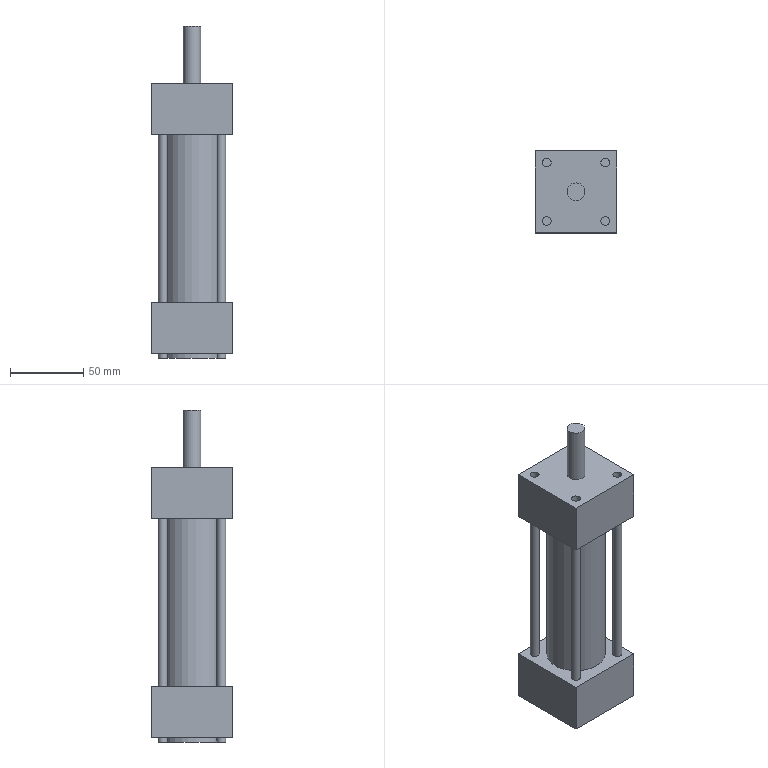Part | NX | features MAIN_BODY 2 | 1 solid | 37 faces | box 56 x 56 x 227 mm | volume 382506 mm3 | plane 22 | cylinder 15 | commonest cylinder face diameters 6.2 x8 6 x4 40 x2 12 x1
STEP:
#1=CARTESIAN_POINT('',(652.5,-160.,-165.));
#2=VERTEX_POINT('',#1);
#3=CARTESIAN_POINT('',(652.5,-140.,-165.));
#4=DIRECTION('',(0.,0.,1.));
#5=DIRECTION('',(0.,-1.,0.));
#6=AXIS2_PLACEMENT_3D('',#3,#4,#5);
#7=CIRCLE('',#6,20.);
#8=EDGE_CURVE('',#2,#2,#7,.T.);
#9=ORIENTED_EDGE('',*,*,#8,.F.);
#10=EDGE_LOOP('',(#9));
#11=FACE_BOUND('',#10,.T.);
#12=CARTESIAN_POINT('',(652.5,-160.,-280.));
#13=VERTEX_POINT('',#12);
#14=CARTESIAN_POINT('',(652.5,-140.,-280.));
#15=DIRECTION('',(0.,0.,1.));
#16=DIRECTION('',(0.,-1.,0.));
#17=AXIS2_PLACEMENT_3D('',#14,#15,#16);
#18=CIRCLE('',#17,20.);
#19=EDGE_CURVE('',#13,#13,#18,.F.);
#20=ORIENTED_EDGE('',*,*,#19,.F.);
#21=EDGE_LOOP('',(#20));
#22=FACE_BOUND('',#21,.T.);
#23=CARTESIAN_POINT('',(652.5,-140.,-315.));
#24=DIRECTION('',(0.,0.,1.));
#25=DIRECTION('',(0.,1.,0.));
#26=AXIS2_PLACEMENT_3D('',#23,#24,#25);
#27=CYLINDRICAL_SURFACE('',#26,20.);
#28=ADVANCED_FACE('',(#11,#22),#27,.T.);
#29=CARTESIAN_POINT('',(632.5,-163.,-130.));
#30=VERTEX_POINT('',#29);
#31=CARTESIAN_POINT('',(632.5,-160.,-130.));
#32=DIRECTION('',(0.,0.,-1.));
#33=DIRECTION('',(0.,-1.,0.));
#34=AXIS2_PLACEMENT_3D('',#31,#32,#33);
#35=CIRCLE('',#34,3.);
#36=EDGE_CURVE('',#30,#30,#35,.T.);
#37=ORIENTED_EDGE('',*,*,#36,.T.);
#38=EDGE_LOOP('',(#37));
#39=FACE_BOUND('',#38,.T.);
#40=CARTESIAN_POINT('',(632.5,-117.,-130.));
#41=VERTEX_POINT('',#40);
#42=CARTESIAN_POINT('',(632.5,-120.,-130.));
#43=DIRECTION('',(0.,0.,1.));
#44=DIRECTION('',(0.,1.,0.));
#45=AXIS2_PLACEMENT_3D('',#42,#43,#44);
#46=CIRCLE('',#45,3.);
#47=EDGE_CURVE('',#41,#41,#46,.T.);
#48=ORIENTED_EDGE('',*,*,#47,.F.);
#49=EDGE_LOOP('',(#48));
#50=FACE_BOUND('',#49,.T.);
#51=CARTESIAN_POINT('',(680.5,-112.,-130.));
#52=VERTEX_POINT('',#51);
#53=CARTESIAN_POINT('',(624.5,-112.,-130.));
#54=VERTEX_POINT('',#53);
#55=CARTESIAN_POINT('',(680.5,-112.,-130.));
#56=DIRECTION('',(-1.,0.,0.));
#57=VECTOR('',#56,1000.);
#58=LINE('',#55,#57);
#59=EDGE_CURVE('',#52,#54,#58,.T.);
#60=ORIENTED_EDGE('',*,*,#59,.T.);
#61=CARTESIAN_POINT('',(624.5,-168.,-130.));
#62=VERTEX_POINT('',#61);
#63=CARTESIAN_POINT('',(624.5,-112.,-130.));
#64=DIRECTION('',(0.,-1.,0.));
#65=VECTOR('',#64,1000.);
#66=LINE('',#63,#65);
#67=EDGE_CURVE('',#54,#62,#66,.T.);
#68=ORIENTED_EDGE('',*,*,#67,.T.);
#69=CARTESIAN_POINT('',(680.5,-168.,-130.));
#70=VERTEX_POINT('',#69);
#71=CARTESIAN_POINT('',(624.5,-168.,-130.));
#72=DIRECTION('',(1.,0.,0.));
#73=VECTOR('',#72,1000.);
#74=LINE('',#71,#73);
#75=EDGE_CURVE('',#62,#70,#74,.T.);
#76=ORIENTED_EDGE('',*,*,#75,.T.);
#77=CARTESIAN_POINT('',(680.5,-168.,-130.));
#78=DIRECTION('',(0.,1.,0.));
#79=VECTOR('',#78,1000.);
#80=LINE('',#77,#79);
#81=EDGE_CURVE('',#70,#52,#80,.T.);
#82=ORIENTED_EDGE('',*,*,#81,.T.);
#83=EDGE_LOOP('',(#60,#68,#76,#82));
#84=FACE_BOUND('',#83,.T.);
#85=CARTESIAN_POINT('',(672.5,-163.,-130.));
#86=VERTEX_POINT('',#85);
#87=CARTESIAN_POINT('',(672.5,-160.,-130.));
#88=DIRECTION('',(0.,0.,1.));
#89=DIRECTION('',(0.,-1.,0.));
#90=AXIS2_PLACEMENT_3D('',#87,#88,#89);
#91=CIRCLE('',#90,3.);
#92=EDGE_CURVE('',#86,#86,#91,.T.);
#93=ORIENTED_EDGE('',*,*,#92,.F.);
#94=EDGE_LOOP('',(#93));
#95=FACE_BOUND('',#94,.T.);
#96=CARTESIAN_POINT('',(672.5,-117.,-130.));
#97=VERTEX_POINT('',#96);
#98=CARTESIAN_POINT('',(672.5,-120.,-130.));
#99=DIRECTION('',(0.,0.,-1.));
#100=DIRECTION('',(0.,1.,0.));
#101=AXIS2_PLACEMENT_3D('',#98,#99,#100);
#102=CIRCLE('',#101,3.);
#103=EDGE_CURVE('',#97,#97,#102,.T.);
#104=ORIENTED_EDGE('',*,*,#103,.T.);
#105=EDGE_LOOP('',(#104));
#106=FACE_BOUND('',#105,.T.);
#107=CARTESIAN_POINT('',(652.5,-146.,-130.));
#108=VERTEX_POINT('',#107);
#109=CARTESIAN_POINT('',(652.5,-140.,-130.));
#110=DIRECTION('',(0.,0.,1.));
#111=DIRECTION('',(0.,-1.,0.));
#112=AXIS2_PLACEMENT_3D('',#109,#110,#111);
#113=CIRCLE('',#112,6.);
#114=EDGE_CURVE('',#108,#108,#113,.F.);
#115=ORIENTED_EDGE('',*,*,#114,.T.);
#116=EDGE_LOOP('',(#115));
#117=FACE_BOUND('',#116,.T.);
#118=CARTESIAN_POINT('',(624.5,-112.,-130.));
#119=DIRECTION('',(0.,0.,-1.));
#120=DIRECTION('',(0.,-1.,0.));
#121=AXIS2_PLACEMENT_3D('',#118,#119,#120);
#122=PLANE('',#121);
#123=ADVANCED_FACE('',(#39,#50,#84,#95,#106,#117),#122,.F.);
#124=ORIENTED_EDGE('',*,*,#59,.F.);
#125=CARTESIAN_POINT('',(680.5,-112.,-165.));
#126=VERTEX_POINT('',#125);
#127=CARTESIAN_POINT('',(680.5,-112.,-165.));
#128=DIRECTION('',(0.,0.,1.));
#129=VECTOR('',#128,1000.);
#130=LINE('',#127,#129);
#131=EDGE_CURVE('',#126,#52,#130,.T.);
#132=ORIENTED_EDGE('',*,*,#131,.F.);
#133=CARTESIAN_POINT('',(624.5,-112.,-165.));
#134=VERTEX_POINT('',#133);
#135=CARTESIAN_POINT('',(680.5,-112.,-165.));
#136=DIRECTION('',(-1.,0.,0.));
#137=VECTOR('',#136,1000.);
#138=LINE('',#135,#137);
#139=EDGE_CURVE('',#126,#134,#138,.T.);
#140=ORIENTED_EDGE('',*,*,#139,.T.);
#141=CARTESIAN_POINT('',(624.5,-112.,-165.));
#142=DIRECTION('',(0.,0.,1.));
#143=VECTOR('',#142,1000.);
#144=LINE('',#141,#143);
#145=EDGE_CURVE('',#134,#54,#144,.T.);
#146=ORIENTED_EDGE('',*,*,#145,.T.);
#147=EDGE_LOOP('',(#124,#132,#140,#146));
#148=FACE_BOUND('',#147,.T.);
#149=CARTESIAN_POINT('',(680.5,-112.,-165.));
#150=DIRECTION('',(0.,-1.,0.));
#151=DIRECTION('',(-1.,0.,0.));
#152=AXIS2_PLACEMENT_3D('',#149,#150,#151);
#153=PLANE('',#152);
#154=ADVANCED_FACE('',(#148),#153,.F.);
#155=ORIENTED_EDGE('',*,*,#67,.F.);
#156=ORIENTED_EDGE('',*,*,#145,.F.);
#157=CARTESIAN_POINT('',(624.5,-168.,-165.));
#158=VERTEX_POINT('',#157);
#159=CARTESIAN_POINT('',(624.5,-112.,-165.));
#160=DIRECTION('',(0.,-1.,0.));
#161=VECTOR('',#160,1000.);
#162=LINE('',#159,#161);
#163=EDGE_CURVE('',#134,#158,#162,.T.);
#164=ORIENTED_EDGE('',*,*,#163,.T.);
#165=CARTESIAN_POINT('',(624.5,-168.,-165.));
#166=DIRECTION('',(0.,0.,1.));
#167=VECTOR('',#166,1000.);
#168=LINE('',#165,#167);
#169=EDGE_CURVE('',#158,#62,#168,.T.);
#170=ORIENTED_EDGE('',*,*,#169,.T.);
#171=EDGE_LOOP('',(#155,#156,#164,#170));
#172=FACE_BOUND('',#171,.T.);
#173=CARTESIAN_POINT('',(624.5,-112.,-165.));
#174=DIRECTION('',(1.,0.,0.));
#175=DIRECTION('',(0.,0.,1.));
#176=AXIS2_PLACEMENT_3D('',#173,#174,#175);
#177=PLANE('',#176);
#178=ADVANCED_FACE('',(#172),#177,.F.);
#179=ORIENTED_EDGE('',*,*,#75,.F.);
#180=ORIENTED_EDGE('',*,*,#169,.F.);
#181=CARTESIAN_POINT('',(680.5,-168.,-165.));
#182=VERTEX_POINT('',#181);
#183=CARTESIAN_POINT('',(624.5,-168.,-165.));
#184=DIRECTION('',(1.,0.,0.));
#185=VECTOR('',#184,1000.);
#186=LINE('',#183,#185);
#187=EDGE_CURVE('',#158,#182,#186,.T.);
#188=ORIENTED_EDGE('',*,*,#187,.T.);
#189=CARTESIAN_POINT('',(680.5,-168.,-165.));
#190=DIRECTION('',(0.,0.,1.));
#191=VECTOR('',#190,1000.);
#192=LINE('',#189,#191);
#193=EDGE_CURVE('',#182,#70,#192,.T.);
#194=ORIENTED_EDGE('',*,*,#193,.T.);
#195=EDGE_LOOP('',(#179,#180,#188,#194));
#196=FACE_BOUND('',#195,.T.);
#197=CARTESIAN_POINT('',(624.5,-168.,-165.));
#198=DIRECTION('',(0.,1.,0.));
#199=DIRECTION('',(0.,0.,-1.));
#200=AXIS2_PLACEMENT_3D('',#197,#198,#199);
#201=PLANE('',#200);
#202=ADVANCED_FACE('',(#196),#201,.F.);
#203=CARTESIAN_POINT('',(632.5,-123.,-165.));
#204=VERTEX_POINT('',#203);
#205=CARTESIAN_POINT('',(632.5,-120.,-165.));
#206=DIRECTION('',(0.,0.,1.));
#207=DIRECTION('',(0.,-1.,0.));
#208=AXIS2_PLACEMENT_3D('',#205,#206,#207);
#209=CIRCLE('',#208,3.);
#210=EDGE_CURVE('',#204,#204,#209,.T.);
#211=ORIENTED_EDGE('',*,*,#210,.F.);
#212=EDGE_LOOP('',(#211));
#213=FACE_BOUND('',#212,.T.);
#214=ORIENTED_EDGE('',*,*,#47,.T.);
#215=EDGE_LOOP('',(#214));
#216=FACE_BOUND('',#215,.T.);
#217=CARTESIAN_POINT('',(632.5,-120.,-165.));
#218=DIRECTION('',(0.,0.,1.));
#219=DIRECTION('',(0.,1.,0.));
#220=AXIS2_PLACEMENT_3D('',#217,#218,#219);
#221=CYLINDRICAL_SURFACE('',#220,3.);
#222=ADVANCED_FACE('',(#213,#216),#221,.F.);
#223=ORIENTED_EDGE('',*,*,#81,.F.);
#224=ORIENTED_EDGE('',*,*,#193,.F.);
#225=CARTESIAN_POINT('',(680.5,-168.,-165.));
#226=DIRECTION('',(0.,1.,0.));
#227=VECTOR('',#226,1000.);
#228=LINE('',#225,#227);
#229=EDGE_CURVE('',#182,#126,#228,.T.);
#230=ORIENTED_EDGE('',*,*,#229,.T.);
#231=ORIENTED_EDGE('',*,*,#131,.T.);
#232=EDGE_LOOP('',(#223,#224,#230,#231));
#233=FACE_BOUND('',#232,.T.);
#234=CARTESIAN_POINT('',(680.5,-168.,-165.));
#235=DIRECTION('',(-1.,0.,0.));
#236=DIRECTION('',(0.,0.,-1.));
#237=AXIS2_PLACEMENT_3D('',#234,#235,#236);
#238=PLANE('',#237);
#239=ADVANCED_FACE('',(#233),#238,.F.);
#240=CARTESIAN_POINT('',(672.5,-163.,-165.));
#241=VERTEX_POINT('',#240);
#242=CARTESIAN_POINT('',(672.5,-160.,-165.));
#243=DIRECTION('',(0.,0.,1.));
#244=DIRECTION('',(0.,-1.,0.));
#245=AXIS2_PLACEMENT_3D('',#242,#243,#244);
#246=CIRCLE('',#245,3.);
#247=EDGE_CURVE('',#241,#241,#246,.T.);
#248=ORIENTED_EDGE('',*,*,#247,.F.);
#249=EDGE_LOOP('',(#248));
#250=FACE_BOUND('',#249,.T.);
#251=ORIENTED_EDGE('',*,*,#92,.T.);
#252=EDGE_LOOP('',(#251));
#253=FACE_BOUND('',#252,.T.);
#254=CARTESIAN_POINT('',(672.5,-160.,-165.));
#255=DIRECTION('',(0.,0.,1.));
#256=DIRECTION('',(0.,1.,0.));
#257=AXIS2_PLACEMENT_3D('',#254,#255,#256);
#258=CYLINDRICAL_SURFACE('',#257,3.);
#259=ADVANCED_FACE('',(#250,#253),#258,.F.);
#260=CARTESIAN_POINT('',(672.5,-117.,-165.));
#261=VERTEX_POINT('',#260);
#262=CARTESIAN_POINT('',(672.5,-120.,-165.));
#263=DIRECTION('',(0.,0.,-1.));
#264=DIRECTION('',(0.,1.,0.));
#265=AXIS2_PLACEMENT_3D('',#262,#263,#264);
#266=CIRCLE('',#265,3.);
#267=EDGE_CURVE('',#261,#261,#266,.T.);
#268=ORIENTED_EDGE('',*,*,#267,.T.);
#269=EDGE_LOOP('',(#268));
#270=FACE_BOUND('',#269,.T.);
#271=ORIENTED_EDGE('',*,*,#103,.F.);
#272=EDGE_LOOP('',(#271));
#273=FACE_BOUND('',#272,.T.);
#274=CARTESIAN_POINT('',(672.5,-120.,-165.));
#275=DIRECTION('',(0.,0.,1.));
#276=DIRECTION('',(0.,1.,0.));
#277=AXIS2_PLACEMENT_3D('',#274,#275,#276);
#278=CYLINDRICAL_SURFACE('',#277,3.);
#279=ADVANCED_FACE('',(#270,#273),#278,.F.);
#280=CARTESIAN_POINT('',(632.5,-163.,-165.));
#281=VERTEX_POINT('',#280);
#282=CARTESIAN_POINT('',(632.5,-160.,-165.));
#283=DIRECTION('',(0.,0.,-1.));
#284=DIRECTION('',(0.,-1.,0.));
#285=AXIS2_PLACEMENT_3D('',#282,#283,#284);
#286=CIRCLE('',#285,3.);
#287=EDGE_CURVE('',#281,#281,#286,.T.);
#288=ORIENTED_EDGE('',*,*,#287,.T.);
#289=EDGE_LOOP('',(#288));
#290=FACE_BOUND('',#289,.T.);
#291=ORIENTED_EDGE('',*,*,#36,.F.);
#292=EDGE_LOOP('',(#291));
#293=FACE_BOUND('',#292,.T.);
#294=CARTESIAN_POINT('',(632.5,-160.,-165.));
#295=DIRECTION('',(0.,0.,1.));
#296=DIRECTION('',(0.,1.,0.));
#297=AXIS2_PLACEMENT_3D('',#294,#295,#296);
#298=CYLINDRICAL_SURFACE('',#297,3.);
#299=ADVANCED_FACE('',(#290,#293),#298,.F.);
#300=CARTESIAN_POINT('',(632.5,-123.1,-165.));
#301=VERTEX_POINT('',#300);
#302=CARTESIAN_POINT('',(632.5,-120.,-165.));
#303=DIRECTION('',(0.,0.,1.));
#304=DIRECTION('',(0.,-1.,0.));
#305=AXIS2_PLACEMENT_3D('',#302,#303,#304);
#306=CIRCLE('',#305,3.1);
#307=EDGE_CURVE('',#301,#301,#306,.T.);
#308=ORIENTED_EDGE('',*,*,#307,.T.);
#309=EDGE_LOOP('',(#308));
#310=FACE_BOUND('',#309,.T.);
#311=CARTESIAN_POINT('',(672.5,-123.1,-165.));
#312=VERTEX_POINT('',#311);
#313=CARTESIAN_POINT('',(672.5,-120.,-165.));
#314=DIRECTION('',(0.,0.,1.));
#315=DIRECTION('',(0.,-1.,0.));
#316=AXIS2_PLACEMENT_3D('',#313,#314,#315);
#317=CIRCLE('',#316,3.1);
#318=EDGE_CURVE('',#312,#312,#317,.T.);
#319=ORIENTED_EDGE('',*,*,#318,.T.);
#320=EDGE_LOOP('',(#319));
#321=FACE_BOUND('',#320,.T.);
#322=CARTESIAN_POINT('',(672.5,-163.1,-165.));
#323=VERTEX_POINT('',#322);
#324=CARTESIAN_POINT('',(672.5,-160.,-165.));
#325=DIRECTION('',(0.,0.,1.));
#326=DIRECTION('',(0.,-1.,0.));
#327=AXIS2_PLACEMENT_3D('',#324,#325,#326);
#328=CIRCLE('',#327,3.1);
#329=EDGE_CURVE('',#323,#323,#328,.T.);
#330=ORIENTED_EDGE('',*,*,#329,.T.);
#331=EDGE_LOOP('',(#330));
#332=FACE_BOUND('',#331,.T.);
#333=CARTESIAN_POINT('',(632.5,-163.1,-165.));
#334=VERTEX_POINT('',#333);
#335=CARTESIAN_POINT('',(632.5,-160.,-165.));
#336=DIRECTION('',(0.,0.,1.));
#337=DIRECTION('',(0.,-1.,0.));
#338=AXIS2_PLACEMENT_3D('',#335,#336,#337);
#339=CIRCLE('',#338,3.1);
#340=EDGE_CURVE('',#334,#334,#339,.T.);
#341=ORIENTED_EDGE('',*,*,#340,.T.);
#342=EDGE_LOOP('',(#341));
#343=FACE_BOUND('',#342,.T.);
#344=ORIENTED_EDGE('',*,*,#8,.T.);
#345=EDGE_LOOP('',(#344));
#346=FACE_BOUND('',#345,.T.);
#347=ORIENTED_EDGE('',*,*,#139,.F.);
#348=ORIENTED_EDGE('',*,*,#229,.F.);
#349=ORIENTED_EDGE('',*,*,#187,.F.);
#350=ORIENTED_EDGE('',*,*,#163,.F.);
#351=EDGE_LOOP('',(#347,#348,#349,#350));
#352=FACE_BOUND('',#351,.T.);
#353=CARTESIAN_POINT('',(624.5,-112.,-165.));
#354=DIRECTION('',(0.,0.,-1.));
#355=DIRECTION('',(0.,-1.,0.));
#356=AXIS2_PLACEMENT_3D('',#353,#354,#355);
#357=PLANE('',#356);
#358=ADVANCED_FACE('',(#310,#321,#332,#343,#346,#352),#357,.T.);
#359=CARTESIAN_POINT('',(652.5,-134.,-91.));
#360=VERTEX_POINT('',#359);
#361=CARTESIAN_POINT('',(652.5,-140.,-91.));
#362=DIRECTION('',(0.,0.,-1.));
#363=DIRECTION('',(0.,1.,0.));
#364=AXIS2_PLACEMENT_3D('',#361,#362,#363);
#365=CIRCLE('',#364,6.);
#366=EDGE_CURVE('',#360,#360,#365,.T.);
#367=ORIENTED_EDGE('',*,*,#366,.F.);
#368=EDGE_LOOP('',(#367));
#369=FACE_BOUND('',#368,.T.);
#370=CARTESIAN_POINT('',(615.,15.,-91.));
#371=DIRECTION('',(0.,0.,1.));
#372=DIRECTION('',(0.,1.,0.));
#373=AXIS2_PLACEMENT_3D('',#370,#371,#372);
#374=PLANE('',#373);
#375=ADVANCED_FACE('',(#369),#374,.T.);
#376=ORIENTED_EDGE('',*,*,#114,.F.);
#377=EDGE_LOOP('',(#376));
#378=FACE_BOUND('',#377,.T.);
#379=ORIENTED_EDGE('',*,*,#366,.T.);
#380=EDGE_LOOP('',(#379));
#381=FACE_BOUND('',#380,.T.);
#382=CARTESIAN_POINT('',(652.5,-140.,-80.));
#383=DIRECTION('',(0.,0.,-1.));
#384=DIRECTION('',(0.,-1.,0.));
#385=AXIS2_PLACEMENT_3D('',#382,#383,#384);
#386=CYLINDRICAL_SURFACE('',#385,6.);
#387=ADVANCED_FACE('',(#378,#381),#386,.T.);
#388=CARTESIAN_POINT('',(624.5,-112.,-280.));
#389=VERTEX_POINT('',#388);
#390=CARTESIAN_POINT('',(624.5,-168.,-280.));
#391=VERTEX_POINT('',#390);
#392=CARTESIAN_POINT('',(624.5,-112.,-280.));
#393=DIRECTION('',(0.,-1.,0.));
#394=VECTOR('',#393,1000.);
#395=LINE('',#392,#394);
#396=EDGE_CURVE('',#389,#391,#395,.T.);
#397=ORIENTED_EDGE('',*,*,#396,.F.);
#398=CARTESIAN_POINT('',(624.5,-112.,-315.));
#399=VERTEX_POINT('',#398);
#400=CARTESIAN_POINT('',(624.5,-112.,-315.));
#401=DIRECTION('',(0.,0.,1.));
#402=VECTOR('',#401,1000.);
#403=LINE('',#400,#402);
#404=EDGE_CURVE('',#399,#389,#403,.T.);
#405=ORIENTED_EDGE('',*,*,#404,.F.);
#406=CARTESIAN_POINT('',(624.5,-168.,-315.));
#407=VERTEX_POINT('',#406);
#408=CARTESIAN_POINT('',(624.5,-112.,-315.));
#409=DIRECTION('',(0.,-1.,0.));
#410=VECTOR('',#409,1000.);
#411=LINE('',#408,#410);
#412=EDGE_CURVE('',#399,#407,#411,.T.);
#413=ORIENTED_EDGE('',*,*,#412,.T.);
#414=CARTESIAN_POINT('',(624.5,-168.,-315.));
#415=DIRECTION('',(0.,0.,1.));
#416=VECTOR('',#415,1000.);
#417=LINE('',#414,#416);
#418=EDGE_CURVE('',#407,#391,#417,.T.);
#419=ORIENTED_EDGE('',*,*,#418,.T.);
#420=EDGE_LOOP('',(#397,#405,#413,#419));
#421=FACE_BOUND('',#420,.T.);
#422=CARTESIAN_POINT('',(624.5,-112.,-315.));
#423=DIRECTION('',(1.,0.,0.));
#424=DIRECTION('',(0.,0.,1.));
#425=AXIS2_PLACEMENT_3D('',#422,#423,#424);
#426=PLANE('',#425);
#427=ADVANCED_FACE('',(#421),#426,.F.);
#428=CARTESIAN_POINT('',(680.5,-168.,-280.));
#429=VERTEX_POINT('',#428);
#430=CARTESIAN_POINT('',(624.5,-168.,-280.));
#431=DIRECTION('',(1.,0.,0.));
#432=VECTOR('',#431,1000.);
#433=LINE('',#430,#432);
#434=EDGE_CURVE('',#391,#429,#433,.T.);
#435=ORIENTED_EDGE('',*,*,#434,.F.);
#436=ORIENTED_EDGE('',*,*,#418,.F.);
#437=CARTESIAN_POINT('',(680.5,-168.,-315.));
#438=VERTEX_POINT('',#437);
#439=CARTESIAN_POINT('',(624.5,-168.,-315.));
#440=DIRECTION('',(1.,0.,0.));
#441=VECTOR('',#440,1000.);
#442=LINE('',#439,#441);
#443=EDGE_CURVE('',#407,#438,#442,.T.);
#444=ORIENTED_EDGE('',*,*,#443,.T.);
#445=CARTESIAN_POINT('',(680.5,-168.,-315.));
#446=DIRECTION('',(0.,0.,1.));
#447=VECTOR('',#446,1000.);
#448=LINE('',#445,#447);
#449=EDGE_CURVE('',#438,#429,#448,.T.);
#450=ORIENTED_EDGE('',*,*,#449,.T.);
#451=EDGE_LOOP('',(#435,#436,#444,#450));
#452=FACE_BOUND('',#451,.T.);
#453=CARTESIAN_POINT('',(624.5,-168.,-315.));
#454=DIRECTION('',(0.,1.,0.));
#455=DIRECTION('',(0.,0.,-1.));
#456=AXIS2_PLACEMENT_3D('',#453,#454,#455);
#457=PLANE('',#456);
#458=ADVANCED_FACE('',(#452),#457,.F.);
#459=CARTESIAN_POINT('',(680.5,-112.,-280.));
#460=VERTEX_POINT('',#459);
#461=CARTESIAN_POINT('',(680.5,-168.,-280.));
#462=DIRECTION('',(0.,1.,0.));
#463=VECTOR('',#462,1000.);
#464=LINE('',#461,#463);
#465=EDGE_CURVE('',#429,#460,#464,.T.);
#466=ORIENTED_EDGE('',*,*,#465,.F.);
#467=ORIENTED_EDGE('',*,*,#449,.F.);
#468=CARTESIAN_POINT('',(680.5,-112.,-315.));
#469=VERTEX_POINT('',#468);
#470=CARTESIAN_POINT('',(680.5,-168.,-315.));
#471=DIRECTION('',(0.,1.,0.));
#472=VECTOR('',#471,1000.);
#473=LINE('',#470,#472);
#474=EDGE_CURVE('',#438,#469,#473,.T.);
#475=ORIENTED_EDGE('',*,*,#474,.T.);
#476=CARTESIAN_POINT('',(680.5,-112.,-315.));
#477=DIRECTION('',(0.,0.,1.));
#478=VECTOR('',#477,1000.);
#479=LINE('',#476,#478);
#480=EDGE_CURVE('',#469,#460,#479,.T.);
#481=ORIENTED_EDGE('',*,*,#480,.T.);
#482=EDGE_LOOP('',(#466,#467,#475,#481));
#483=FACE_BOUND('',#482,.T.);
#484=CARTESIAN_POINT('',(680.5,-168.,-315.));
#485=DIRECTION('',(-1.,0.,0.));
#486=DIRECTION('',(0.,0.,-1.));
#487=AXIS2_PLACEMENT_3D('',#484,#485,#486);
#488=PLANE('',#487);
#489=ADVANCED_FACE('',(#483),#488,.F.);
#490=CARTESIAN_POINT('',(680.5,-112.,-280.));
#491=DIRECTION('',(-1.,0.,0.));
#492=VECTOR('',#491,1000.);
#493=LINE('',#490,#492);
#494=EDGE_CURVE('',#460,#389,#493,.T.);
#495=ORIENTED_EDGE('',*,*,#494,.F.);
#496=ORIENTED_EDGE('',*,*,#480,.F.);
#497=CARTESIAN_POINT('',(680.5,-112.,-315.));
#498=DIRECTION('',(-1.,0.,0.));
#499=VECTOR('',#498,1000.);
#500=LINE('',#497,#499);
#501=EDGE_CURVE('',#469,#399,#500,.T.);
#502=ORIENTED_EDGE('',*,*,#501,.T.);
#503=ORIENTED_EDGE('',*,*,#404,.T.);
#504=EDGE_LOOP('',(#495,#496,#502,#503));
#505=FACE_BOUND('',#504,.T.);
#506=CARTESIAN_POINT('',(680.5,-112.,-315.));
#507=DIRECTION('',(0.,-1.,0.));
#508=DIRECTION('',(-1.,0.,0.));
#509=AXIS2_PLACEMENT_3D('',#506,#507,#508);
#510=PLANE('',#509);
#511=ADVANCED_FACE('',(#505),#510,.F.);
#512=CARTESIAN_POINT('',(632.5,-123.1,-315.));
#513=VERTEX_POINT('',#512);
#514=CARTESIAN_POINT('',(632.5,-120.,-315.));
#515=DIRECTION('',(0.,0.,1.));
#516=DIRECTION('',(0.,-1.,0.));
#517=AXIS2_PLACEMENT_3D('',#514,#515,#516);
#518=CIRCLE('',#517,3.1);
#519=EDGE_CURVE('',#513,#513,#518,.T.);
#520=ORIENTED_EDGE('',*,*,#519,.T.);
#521=EDGE_LOOP('',(#520));
#522=FACE_BOUND('',#521,.T.);
#523=CARTESIAN_POINT('',(672.5,-123.1,-315.));
#524=VERTEX_POINT('',#523);
#525=CARTESIAN_POINT('',(672.5,-120.,-315.));
#526=DIRECTION('',(0.,0.,1.));
#527=DIRECTION('',(0.,-1.,0.));
#528=AXIS2_PLACEMENT_3D('',#525,#526,#527);
#529=CIRCLE('',#528,3.1);
#530=EDGE_CURVE('',#524,#524,#529,.T.);
#531=ORIENTED_EDGE('',*,*,#530,.T.);
#532=EDGE_LOOP('',(#531));
#533=FACE_BOUND('',#532,.T.);
#534=CARTESIAN_POINT('',(672.5,-163.1,-315.));
#535=VERTEX_POINT('',#534);
#536=CARTESIAN_POINT('',(672.5,-160.,-315.));
#537=DIRECTION('',(0.,0.,1.));
#538=DIRECTION('',(0.,-1.,0.));
#539=AXIS2_PLACEMENT_3D('',#536,#537,#538);
#540=CIRCLE('',#539,3.1);
#541=EDGE_CURVE('',#535,#535,#540,.T.);
#542=ORIENTED_EDGE('',*,*,#541,.T.);
#543=EDGE_LOOP('',(#542));
#544=FACE_BOUND('',#543,.T.);
#545=CARTESIAN_POINT('',(632.5,-163.1,-315.));
#546=VERTEX_POINT('',#545);
#547=CARTESIAN_POINT('',(632.5,-160.,-315.));
#548=DIRECTION('',(0.,0.,1.));
#549=DIRECTION('',(0.,-1.,0.));
#550=AXIS2_PLACEMENT_3D('',#547,#548,#549);
#551=CIRCLE('',#550,3.1);
#552=EDGE_CURVE('',#546,#546,#551,.T.);
#553=ORIENTED_EDGE('',*,*,#552,.T.);
#554=EDGE_LOOP('',(#553));
#555=FACE_BOUND('',#554,.T.);
#556=CARTESIAN_POINT('',(652.5,-160.,-315.));
#557=VERTEX_POINT('',#556);
#558=CARTESIAN_POINT('',(652.5,-140.,-315.));
#559=DIRECTION('',(0.,0.,1.));
#560=DIRECTION('',(0.,-1.,0.));
#561=AXIS2_PLACEMENT_3D('',#558,#559,#560);
#562=CIRCLE('',#561,20.);
#563=EDGE_CURVE('',#557,#557,#562,.F.);
#564=ORIENTED_EDGE('',*,*,#563,.F.);
#565=EDGE_LOOP('',(#564));
#566=FACE_BOUND('',#565,.T.);
#567=ORIENTED_EDGE('',*,*,#412,.F.);
#568=ORIENTED_EDGE('',*,*,#501,.F.);
#569=ORIENTED_EDGE('',*,*,#474,.F.);
#570=ORIENTED_EDGE('',*,*,#443,.F.);
#571=EDGE_LOOP('',(#567,#568,#569,#570));
#572=FACE_BOUND('',#571,.T.);
#573=CARTESIAN_POINT('',(624.5,-168.,-315.));
#574=DIRECTION('',(0.,0.,-1.));
#575=DIRECTION('',(0.,-1.,0.));
#576=AXIS2_PLACEMENT_3D('',#573,#574,#575);
#577=PLANE('',#576);
#578=ADVANCED_FACE('',(#522,#533,#544,#555,#566,#572),#577,.T.);
#579=CARTESIAN_POINT('',(632.5,-123.1,-280.));
#580=VERTEX_POINT('',#579);
#581=CARTESIAN_POINT('',(632.5,-120.,-280.));
#582=DIRECTION('',(0.,0.,1.));
#583=DIRECTION('',(0.,-1.,0.));
#584=AXIS2_PLACEMENT_3D('',#581,#582,#583);
#585=CIRCLE('',#584,3.1);
#586=EDGE_CURVE('',#580,#580,#585,.T.);
#587=ORIENTED_EDGE('',*,*,#586,.F.);
#588=EDGE_LOOP('',(#587));
#589=FACE_BOUND('',#588,.T.);
#590=CARTESIAN_POINT('',(672.5,-123.1,-280.));
#591=VERTEX_POINT('',#590);
#592=CARTESIAN_POINT('',(672.5,-120.,-280.));
#593=DIRECTION('',(0.,0.,1.));
#594=DIRECTION('',(0.,-1.,0.));
#595=AXIS2_PLACEMENT_3D('',#592,#593,#594);
#596=CIRCLE('',#595,3.1);
#597=EDGE_CURVE('',#591,#591,#596,.T.);
#598=ORIENTED_EDGE('',*,*,#597,.F.);
#599=EDGE_LOOP('',(#598));
#600=FACE_BOUND('',#599,.T.);
#601=CARTESIAN_POINT('',(672.5,-163.1,-280.));
#602=VERTEX_POINT('',#601);
#603=CARTESIAN_POINT('',(672.5,-160.,-280.));
#604=DIRECTION('',(0.,0.,1.));
#605=DIRECTION('',(0.,-1.,0.));
#606=AXIS2_PLACEMENT_3D('',#603,#604,#605);
#607=CIRCLE('',#606,3.1);
#608=EDGE_CURVE('',#602,#602,#607,.T.);
#609=ORIENTED_EDGE('',*,*,#608,.F.);
#610=EDGE_LOOP('',(#609));
#611=FACE_BOUND('',#610,.T.);
#612=CARTESIAN_POINT('',(632.5,-163.1,-280.));
#613=VERTEX_POINT('',#612);
#614=CARTESIAN_POINT('',(632.5,-160.,-280.));
#615=DIRECTION('',(0.,0.,1.));
#616=DIRECTION('',(0.,-1.,0.));
#617=AXIS2_PLACEMENT_3D('',#614,#615,#616);
#618=CIRCLE('',#617,3.1);
#619=EDGE_CURVE('',#613,#613,#618,.T.);
#620=ORIENTED_EDGE('',*,*,#619,.F.);
#621=EDGE_LOOP('',(#620));
#622=FACE_BOUND('',#621,.T.);
#623=ORIENTED_EDGE('',*,*,#19,.T.);
#624=EDGE_LOOP('',(#623));
#625=FACE_BOUND('',#624,.T.);
#626=ORIENTED_EDGE('',*,*,#396,.T.);
#627=ORIENTED_EDGE('',*,*,#434,.T.);
#628=ORIENTED_EDGE('',*,*,#465,.T.);
#629=ORIENTED_EDGE('',*,*,#494,.T.);
#630=EDGE_LOOP('',(#626,#627,#628,#629));
#631=FACE_BOUND('',#630,.T.);
#632=CARTESIAN_POINT('',(624.5,-168.,-280.));
#633=DIRECTION('',(0.,0.,-1.));
#634=DIRECTION('',(0.,-1.,0.));
#635=AXIS2_PLACEMENT_3D('',#632,#633,#634);
#636=PLANE('',#635);
#637=ADVANCED_FACE('',(#589,#600,#611,#622,#625,#631),#636,.F.);
#638=CARTESIAN_POINT('',(652.5,-120.,-318.));
#639=VERTEX_POINT('',#638);
#640=CARTESIAN_POINT('',(652.5,-140.,-318.));
#641=DIRECTION('',(0.,0.,-1.));
#642=DIRECTION('',(0.,1.,0.));
#643=AXIS2_PLACEMENT_3D('',#640,#641,#642);
#644=CIRCLE('',#643,20.);
#645=EDGE_CURVE('',#639,#639,#644,.T.);
#646=ORIENTED_EDGE('',*,*,#645,.T.);
#647=EDGE_LOOP('',(#646));
#648=FACE_BOUND('',#647,.T.);
#649=CARTESIAN_POINT('',(652.5,-140.,-318.));
#650=DIRECTION('',(0.,0.,1.));
#651=DIRECTION('',(0.,1.,0.));
#652=AXIS2_PLACEMENT_3D('',#649,#650,#651);
#653=PLANE('',#652);
#654=ADVANCED_FACE('',(#648),#653,.F.);
#655=ORIENTED_EDGE('',*,*,#563,.T.);
#656=EDGE_LOOP('',(#655));
#657=FACE_BOUND('',#656,.T.);
#658=ORIENTED_EDGE('',*,*,#645,.F.);
#659=EDGE_LOOP('',(#658));
#660=FACE_BOUND('',#659,.T.);
#661=CARTESIAN_POINT('',(652.5,-140.,-315.));
#662=DIRECTION('',(0.,0.,1.));
#663=DIRECTION('',(0.,1.,0.));
#664=AXIS2_PLACEMENT_3D('',#661,#662,#663);
#665=CYLINDRICAL_SURFACE('',#664,20.);
#666=ADVANCED_FACE('',(#657,#660),#665,.T.);
#667=ORIENTED_EDGE('',*,*,#340,.F.);
#668=EDGE_LOOP('',(#667));
#669=FACE_BOUND('',#668,.T.);
#670=ORIENTED_EDGE('',*,*,#619,.T.);
#671=EDGE_LOOP('',(#670));
#672=FACE_BOUND('',#671,.T.);
#673=CARTESIAN_POINT('',(632.5,-160.,-80.));
#674=DIRECTION('',(0.,0.,-1.));
#675=DIRECTION('',(0.,-1.,0.));
#676=AXIS2_PLACEMENT_3D('',#673,#674,#675);
#677=CYLINDRICAL_SURFACE('',#676,3.1);
#678=ADVANCED_FACE('',(#669,#672),#677,.T.);
#679=CARTESIAN_POINT('',(632.5,-156.9,-318.));
#680=VERTEX_POINT('',#679);
#681=CARTESIAN_POINT('',(632.5,-160.,-318.));
#682=DIRECTION('',(0.,0.,-1.));
#683=DIRECTION('',(0.,1.,0.));
#684=AXIS2_PLACEMENT_3D('',#681,#682,#683);
#685=CIRCLE('',#684,3.1);
#686=EDGE_CURVE('',#680,#680,#685,.F.);
#687=ORIENTED_EDGE('',*,*,#686,.F.);
#688=EDGE_LOOP('',(#687));
#689=FACE_BOUND('',#688,.T.);
#690=CARTESIAN_POINT('',(652.5,-140.,-318.));
#691=DIRECTION('',(0.,0.,1.));
#692=DIRECTION('',(0.,1.,0.));
#693=AXIS2_PLACEMENT_3D('',#690,#691,#692);
#694=PLANE('',#693);
#695=ADVANCED_FACE('',(#689),#694,.F.);
#696=ORIENTED_EDGE('',*,*,#552,.F.);
#697=EDGE_LOOP('',(#696));
#698=FACE_BOUND('',#697,.T.);
#699=ORIENTED_EDGE('',*,*,#686,.T.);
#700=EDGE_LOOP('',(#699));
#701=FACE_BOUND('',#700,.T.);
#702=CARTESIAN_POINT('',(632.5,-160.,-80.));
#703=DIRECTION('',(0.,0.,-1.));
#704=DIRECTION('',(0.,-1.,0.));
#705=AXIS2_PLACEMENT_3D('',#702,#703,#704);
#706=CYLINDRICAL_SURFACE('',#705,3.1);
#707=ADVANCED_FACE('',(#698,#701),#706,.T.);
#708=ORIENTED_EDGE('',*,*,#287,.F.);
#709=EDGE_LOOP('',(#708));
#710=FACE_BOUND('',#709,.T.);
#711=CARTESIAN_POINT('',(584.5,-112.,-165.));
#712=DIRECTION('',(0.,0.,-1.));
#713=DIRECTION('',(0.,-1.,0.));
#714=AXIS2_PLACEMENT_3D('',#711,#712,#713);
#715=PLANE('',#714);
#716=ADVANCED_FACE('',(#710),#715,.F.);
#717=ORIENTED_EDGE('',*,*,#329,.F.);
#718=EDGE_LOOP('',(#717));
#719=FACE_BOUND('',#718,.T.);
#720=ORIENTED_EDGE('',*,*,#608,.T.);
#721=EDGE_LOOP('',(#720));
#722=FACE_BOUND('',#721,.T.);
#723=CARTESIAN_POINT('',(672.5,-160.,-80.));
#724=DIRECTION('',(0.,0.,-1.));
#725=DIRECTION('',(0.,-1.,0.));
#726=AXIS2_PLACEMENT_3D('',#723,#724,#725);
#727=CYLINDRICAL_SURFACE('',#726,3.1);
#728=ADVANCED_FACE('',(#719,#722),#727,.T.);
#729=CARTESIAN_POINT('',(672.5,-156.9,-318.));
#730=VERTEX_POINT('',#729);
#731=CARTESIAN_POINT('',(672.5,-160.,-318.));
#732=DIRECTION('',(0.,0.,-1.));
#733=DIRECTION('',(0.,1.,0.));
#734=AXIS2_PLACEMENT_3D('',#731,#732,#733);
#735=CIRCLE('',#734,3.1);
#736=EDGE_CURVE('',#730,#730,#735,.F.);
#737=ORIENTED_EDGE('',*,*,#736,.F.);
#738=EDGE_LOOP('',(#737));
#739=FACE_BOUND('',#738,.T.);
#740=CARTESIAN_POINT('',(652.5,-140.,-318.));
#741=DIRECTION('',(0.,0.,1.));
#742=DIRECTION('',(0.,1.,0.));
#743=AXIS2_PLACEMENT_3D('',#740,#741,#742);
#744=PLANE('',#743);
#745=ADVANCED_FACE('',(#739),#744,.F.);
#746=ORIENTED_EDGE('',*,*,#541,.F.);
#747=EDGE_LOOP('',(#746));
#748=FACE_BOUND('',#747,.T.);
#749=ORIENTED_EDGE('',*,*,#736,.T.);
#750=EDGE_LOOP('',(#749));
#751=FACE_BOUND('',#750,.T.);
#752=CARTESIAN_POINT('',(672.5,-160.,-80.));
#753=DIRECTION('',(0.,0.,-1.));
#754=DIRECTION('',(0.,-1.,0.));
#755=AXIS2_PLACEMENT_3D('',#752,#753,#754);
#756=CYLINDRICAL_SURFACE('',#755,3.1);
#757=ADVANCED_FACE('',(#748,#751),#756,.T.);
#758=ORIENTED_EDGE('',*,*,#247,.T.);
#759=EDGE_LOOP('',(#758));
#760=FACE_BOUND('',#759,.T.);
#761=CARTESIAN_POINT('',(624.5,-112.,-165.));
#762=DIRECTION('',(0.,0.,-1.));
#763=DIRECTION('',(0.,-1.,0.));
#764=AXIS2_PLACEMENT_3D('',#761,#762,#763);
#765=PLANE('',#764);
#766=ADVANCED_FACE('',(#760),#765,.F.);
#767=ORIENTED_EDGE('',*,*,#318,.F.);
#768=EDGE_LOOP('',(#767));
#769=FACE_BOUND('',#768,.T.);
#770=ORIENTED_EDGE('',*,*,#597,.T.);
#771=EDGE_LOOP('',(#770));
#772=FACE_BOUND('',#771,.T.);
#773=CARTESIAN_POINT('',(672.5,-120.,-80.));
#774=DIRECTION('',(0.,0.,-1.));
#775=DIRECTION('',(0.,-1.,0.));
#776=AXIS2_PLACEMENT_3D('',#773,#774,#775);
#777=CYLINDRICAL_SURFACE('',#776,3.1);
#778=ADVANCED_FACE('',(#769,#772),#777,.T.);
#779=CARTESIAN_POINT('',(672.5,-116.9,-318.));
#780=VERTEX_POINT('',#779);
#781=CARTESIAN_POINT('',(672.5,-120.,-318.));
#782=DIRECTION('',(0.,0.,-1.));
#783=DIRECTION('',(0.,1.,0.));
#784=AXIS2_PLACEMENT_3D('',#781,#782,#783);
#785=CIRCLE('',#784,3.1);
#786=EDGE_CURVE('',#780,#780,#785,.F.);
#787=ORIENTED_EDGE('',*,*,#786,.F.);
#788=EDGE_LOOP('',(#787));
#789=FACE_BOUND('',#788,.T.);
#790=CARTESIAN_POINT('',(652.5,-140.,-318.));
#791=DIRECTION('',(0.,0.,1.));
#792=DIRECTION('',(0.,1.,0.));
#793=AXIS2_PLACEMENT_3D('',#790,#791,#792);
#794=PLANE('',#793);
#795=ADVANCED_FACE('',(#789),#794,.F.);
#796=ORIENTED_EDGE('',*,*,#530,.F.);
#797=EDGE_LOOP('',(#796));
#798=FACE_BOUND('',#797,.T.);
#799=ORIENTED_EDGE('',*,*,#786,.T.);
#800=EDGE_LOOP('',(#799));
#801=FACE_BOUND('',#800,.T.);
#802=CARTESIAN_POINT('',(672.5,-120.,-80.));
#803=DIRECTION('',(0.,0.,-1.));
#804=DIRECTION('',(0.,-1.,0.));
#805=AXIS2_PLACEMENT_3D('',#802,#803,#804);
#806=CYLINDRICAL_SURFACE('',#805,3.1);
#807=ADVANCED_FACE('',(#798,#801),#806,.T.);
#808=ORIENTED_EDGE('',*,*,#267,.F.);
#809=EDGE_LOOP('',(#808));
#810=FACE_BOUND('',#809,.T.);
#811=CARTESIAN_POINT('',(624.5,-72.,-165.));
#812=DIRECTION('',(0.,0.,-1.));
#813=DIRECTION('',(0.,-1.,0.));
#814=AXIS2_PLACEMENT_3D('',#811,#812,#813);
#815=PLANE('',#814);
#816=ADVANCED_FACE('',(#810),#815,.F.);
#817=ORIENTED_EDGE('',*,*,#307,.F.);
#818=EDGE_LOOP('',(#817));
#819=FACE_BOUND('',#818,.T.);
#820=ORIENTED_EDGE('',*,*,#586,.T.);
#821=EDGE_LOOP('',(#820));
#822=FACE_BOUND('',#821,.T.);
#823=CARTESIAN_POINT('',(632.5,-120.,-80.));
#824=DIRECTION('',(0.,0.,-1.));
#825=DIRECTION('',(0.,-1.,0.));
#826=AXIS2_PLACEMENT_3D('',#823,#824,#825);
#827=CYLINDRICAL_SURFACE('',#826,3.1);
#828=ADVANCED_FACE('',(#819,#822),#827,.T.);
#829=CARTESIAN_POINT('',(632.5,-116.9,-318.));
#830=VERTEX_POINT('',#829);
#831=CARTESIAN_POINT('',(632.5,-120.,-318.));
#832=DIRECTION('',(0.,0.,-1.));
#833=DIRECTION('',(0.,1.,0.));
#834=AXIS2_PLACEMENT_3D('',#831,#832,#833);
#835=CIRCLE('',#834,3.1);
#836=EDGE_CURVE('',#830,#830,#835,.F.);
#837=ORIENTED_EDGE('',*,*,#836,.F.);
#838=EDGE_LOOP('',(#837));
#839=FACE_BOUND('',#838,.T.);
#840=CARTESIAN_POINT('',(652.5,-140.,-318.));
#841=DIRECTION('',(0.,0.,1.));
#842=DIRECTION('',(0.,1.,0.));
#843=AXIS2_PLACEMENT_3D('',#840,#841,#842);
#844=PLANE('',#843);
#845=ADVANCED_FACE('',(#839),#844,.F.);
#846=ORIENTED_EDGE('',*,*,#519,.F.);
#847=EDGE_LOOP('',(#846));
#848=FACE_BOUND('',#847,.T.);
#849=ORIENTED_EDGE('',*,*,#836,.T.);
#850=EDGE_LOOP('',(#849));
#851=FACE_BOUND('',#850,.T.);
#852=CARTESIAN_POINT('',(632.5,-120.,-80.));
#853=DIRECTION('',(0.,0.,-1.));
#854=DIRECTION('',(0.,-1.,0.));
#855=AXIS2_PLACEMENT_3D('',#852,#853,#854);
#856=CYLINDRICAL_SURFACE('',#855,3.1);
#857=ADVANCED_FACE('',(#848,#851),#856,.T.);
#858=ORIENTED_EDGE('',*,*,#210,.T.);
#859=EDGE_LOOP('',(#858));
#860=FACE_BOUND('',#859,.T.);
#861=CARTESIAN_POINT('',(584.5,-72.,-165.));
#862=DIRECTION('',(0.,0.,-1.));
#863=DIRECTION('',(0.,-1.,0.));
#864=AXIS2_PLACEMENT_3D('',#861,#862,#863);
#865=PLANE('',#864);
#866=ADVANCED_FACE('',(#860),#865,.F.);
#867=CLOSED_SHELL('',(#28,#123,#154,#178,#202,#222,#239,#259,#279,#299,#358,#375,#387,#427,#458,#489,#511,#578,#637,#654,#666,#678,#695,#707,#716,#728,#745,#757,#766,#778,#795,#807,#816,#828,#845,#857,#866));
#868=MANIFOLD_SOLID_BREP('',#867);
#869=(LENGTH_UNIT()NAMED_UNIT(*)SI_UNIT(.MILLI.,.METRE.));
#870=UNCERTAINTY_MEASURE_WITH_UNIT(LENGTH_MEASURE(0.00001),#869,'','');
#871=(NAMED_UNIT(*)PLANE_ANGLE_UNIT()SI_UNIT($,.RADIAN.));
#872=(NAMED_UNIT(*)SI_UNIT($,.STERADIAN.)SOLID_ANGLE_UNIT());
#873=(GEOMETRIC_REPRESENTATION_CONTEXT(3)GLOBAL_UNCERTAINTY_ASSIGNED_CONTEXT((#870))GLOBAL_UNIT_ASSIGNED_CONTEXT((#869,#871,#872))REPRESENTATION_CONTEXT('',''));
#874=ADVANCED_BREP_SHAPE_REPRESENTATION('',(#868),#873);